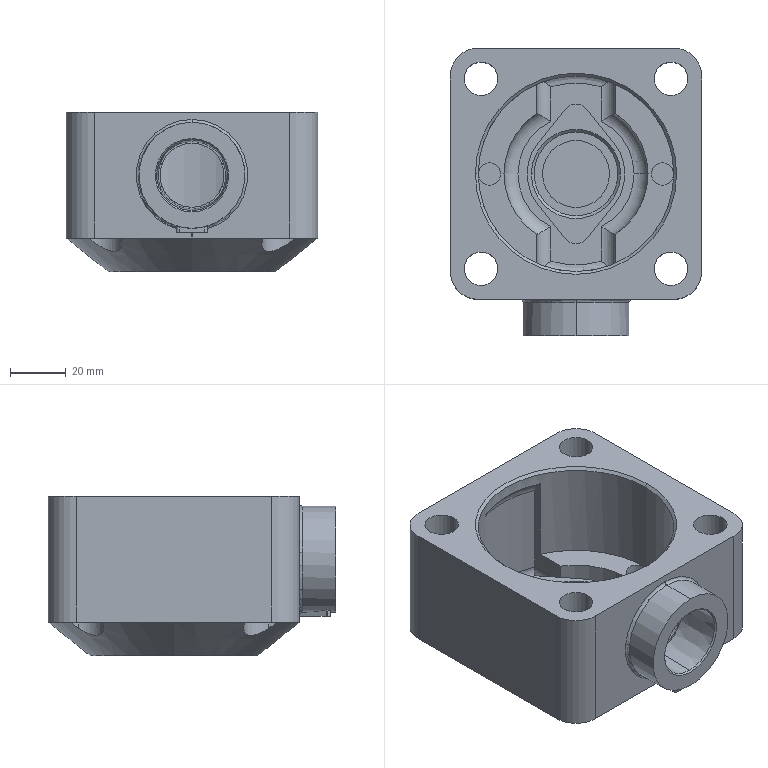Part | SolidWorks | features ICE 13, Fillet 3, 3DProfileFeature 1, Chamfer 1, CirPattern 1, Extrusion 1, HoleWzd 1, Revolution 1 | 1 solid | 110 faces | box 90 x 103 x 57 mm | volume 228367 mm3 | cylinder 51 | plane 40 | cone 10 | torus 9 | commonest cylinder face diameters 12 x8 18 x8 10 x6 8 x4 20 x4 2 x3